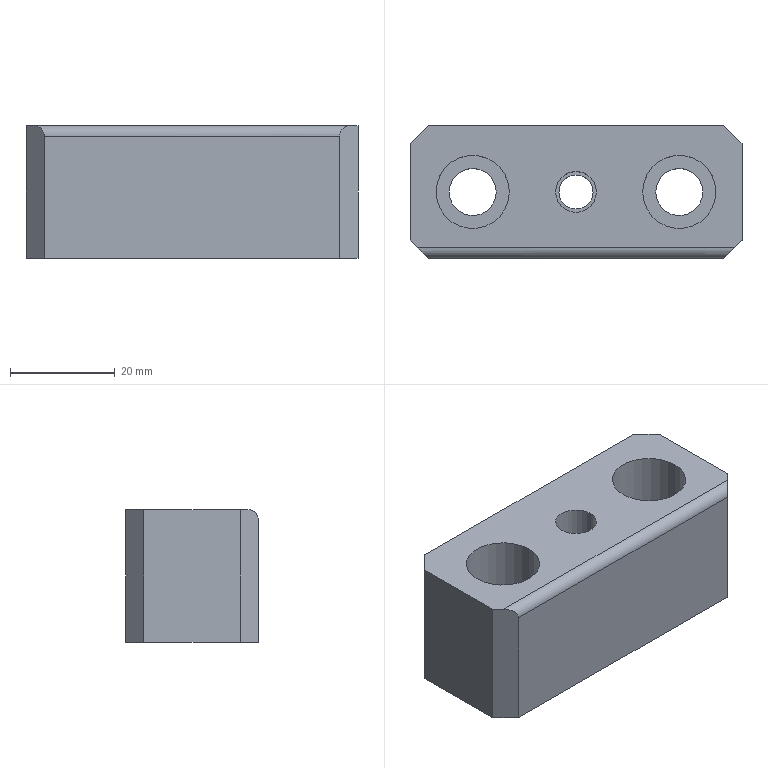Part | STEP file | 1_id1526_x_t | 1 solid | 26 faces | box 63.5 x 25.4 x 25.4 mm | volume 33278 mm3 | plane 13 | cylinder 13 | commonest cylinder face diameters 9 x4 14 x4 6.528 x2 7.8 x2 4 x1